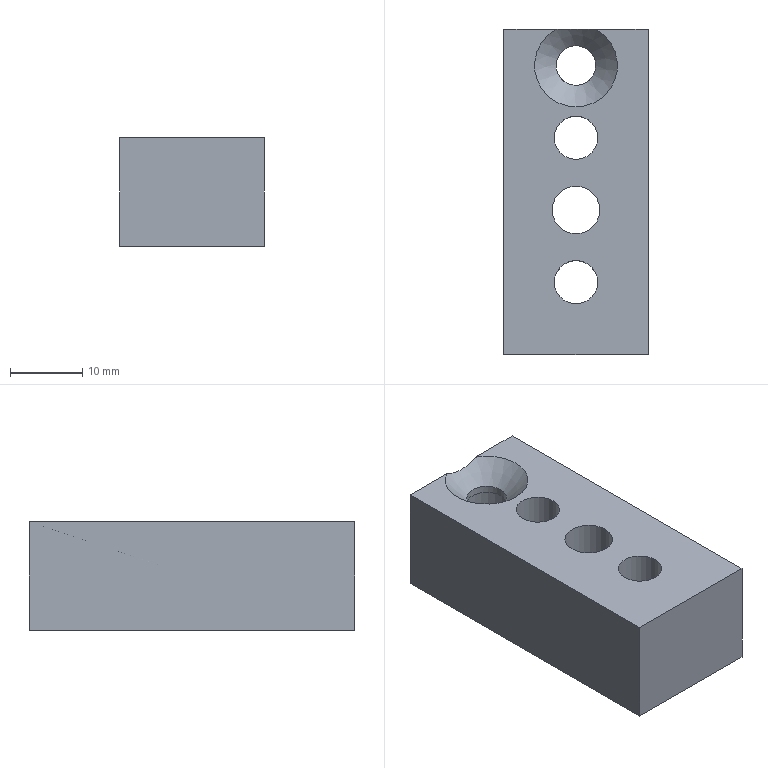Part | NX | features BREP 1 | 1 solid | 15 faces | box 20 x 45 x 15 mm | volume 10997 mm3 | plane 8 | cylinder 6 | cone 1 | commonest cylinder face diameters 6 x2 5.5 x1 6.6 x1 8 x1 11 x1
STEP:
#1=CARTESIAN_POINT('',(-3.,7.5,7.5));
#2=VERTEX_POINT('',#1);
#3=CARTESIAN_POINT('',(0.,7.5,7.5));
#4=DIRECTION('',(0.,0.,-1.));
#5=DIRECTION('',(-1.,0.,0.));
#6=AXIS2_PLACEMENT_3D('',#3,#4,#5);
#7=CIRCLE('',#6,3.);
#8=EDGE_CURVE('',#2,#2,#7,.T.);
#9=ORIENTED_EDGE('',*,*,#8,.T.);
#10=EDGE_LOOP('',(#9));
#11=FACE_BOUND('',#10,.T.);
#12=CARTESIAN_POINT('',(-3.,-12.5,7.5));
#13=VERTEX_POINT('',#12);
#14=CARTESIAN_POINT('',(0.,-12.5,7.5));
#15=DIRECTION('',(0.,0.,-1.));
#16=DIRECTION('',(-1.,0.,0.));
#17=AXIS2_PLACEMENT_3D('',#14,#15,#16);
#18=CIRCLE('',#17,3.);
#19=EDGE_CURVE('',#13,#13,#18,.T.);
#20=ORIENTED_EDGE('',*,*,#19,.T.);
#21=EDGE_LOOP('',(#20));
#22=FACE_BOUND('',#21,.T.);
#23=CARTESIAN_POINT('',(-3.3,-2.5,7.5));
#24=VERTEX_POINT('',#23);
#25=CARTESIAN_POINT('',(0.,-2.5,7.5));
#26=DIRECTION('',(0.,0.,-1.));
#27=DIRECTION('',(-1.,0.,0.));
#28=AXIS2_PLACEMENT_3D('',#25,#26,#27);
#29=CIRCLE('',#28,3.3);
#30=EDGE_CURVE('',#24,#24,#29,.T.);
#31=ORIENTED_EDGE('',*,*,#30,.T.);
#32=EDGE_LOOP('',(#31));
#33=FACE_BOUND('',#32,.T.);
#34=CARTESIAN_POINT('',(-2.809,22.5,7.5));
#35=VERTEX_POINT('',#34);
#36=CARTESIAN_POINT('',(2.809,22.5,7.5));
#37=VERTEX_POINT('',#36);
#38=CARTESIAN_POINT('',(0.,17.5,7.5));
#39=DIRECTION('',(0.,0.,1.));
#40=DIRECTION('',(1.,0.,0.));
#41=AXIS2_PLACEMENT_3D('',#38,#39,#40);
#42=CIRCLE('',#41,5.735);
#43=EDGE_CURVE('',#35,#37,#42,.T.);
#44=ORIENTED_EDGE('',*,*,#43,.F.);
#45=CARTESIAN_POINT('',(-10.,22.5,7.5));
#46=VERTEX_POINT('',#45);
#47=CARTESIAN_POINT('',(-10.,22.5,7.5));
#48=DIRECTION('',(-1.,0.,0.));
#49=VECTOR('',#48,1000.);
#50=LINE('',#47,#49);
#51=EDGE_CURVE('',#35,#46,#50,.T.);
#52=ORIENTED_EDGE('',*,*,#51,.T.);
#53=CARTESIAN_POINT('',(-10.,-22.5,7.5));
#54=VERTEX_POINT('',#53);
#55=CARTESIAN_POINT('',(-10.,-22.5,7.5));
#56=DIRECTION('',(0.,-1.,0.));
#57=VECTOR('',#56,1000.);
#58=LINE('',#55,#57);
#59=EDGE_CURVE('',#46,#54,#58,.T.);
#60=ORIENTED_EDGE('',*,*,#59,.T.);
#61=CARTESIAN_POINT('',(10.,-22.5,7.5));
#62=VERTEX_POINT('',#61);
#63=CARTESIAN_POINT('',(-10.,-22.5,7.5));
#64=DIRECTION('',(1.,0.,0.));
#65=VECTOR('',#64,1000.);
#66=LINE('',#63,#65);
#67=EDGE_CURVE('',#54,#62,#66,.T.);
#68=ORIENTED_EDGE('',*,*,#67,.T.);
#69=CARTESIAN_POINT('',(10.,22.5,7.5));
#70=VERTEX_POINT('',#69);
#71=CARTESIAN_POINT('',(10.,-22.5,7.5));
#72=DIRECTION('',(0.,1.,0.));
#73=VECTOR('',#72,1000.);
#74=LINE('',#71,#73);
#75=EDGE_CURVE('',#62,#70,#74,.T.);
#76=ORIENTED_EDGE('',*,*,#75,.T.);
#77=CARTESIAN_POINT('',(-10.,22.5,7.5));
#78=DIRECTION('',(-1.,0.,0.));
#79=VECTOR('',#78,1000.);
#80=LINE('',#77,#79);
#81=EDGE_CURVE('',#70,#37,#80,.T.);
#82=ORIENTED_EDGE('',*,*,#81,.T.);
#83=EDGE_LOOP('',(#44,#52,#60,#68,#76,#82));
#84=FACE_BOUND('',#83,.T.);
#85=CARTESIAN_POINT('',(0.,0.,7.5));
#86=DIRECTION('',(0.,0.,-1.));
#87=DIRECTION('',(1.,0.,0.));
#88=AXIS2_PLACEMENT_3D('',#85,#86,#87);
#89=PLANE('',#88);
#90=ADVANCED_FACE('',(#11,#22,#33,#84),#89,.F.);
#91=CARTESIAN_POINT('',(10.,-22.5,-7.5));
#92=VERTEX_POINT('',#91);
#93=CARTESIAN_POINT('',(10.,22.5,-7.5));
#94=VERTEX_POINT('',#93);
#95=CARTESIAN_POINT('',(10.,-22.5,-7.5));
#96=DIRECTION('',(0.,1.,0.));
#97=VECTOR('',#96,1000.);
#98=LINE('',#95,#97);
#99=EDGE_CURVE('',#92,#94,#98,.T.);
#100=ORIENTED_EDGE('',*,*,#99,.T.);
#101=CARTESIAN_POINT('',(10.,22.5,7.5));
#102=DIRECTION('',(0.,0.,-1.));
#103=VECTOR('',#102,1000.);
#104=LINE('',#101,#103);
#105=EDGE_CURVE('',#70,#94,#104,.T.);
#106=ORIENTED_EDGE('',*,*,#105,.F.);
#107=ORIENTED_EDGE('',*,*,#75,.F.);
#108=CARTESIAN_POINT('',(10.,-22.5,7.5));
#109=DIRECTION('',(0.,0.,-1.));
#110=VECTOR('',#109,1000.);
#111=LINE('',#108,#110);
#112=EDGE_CURVE('',#62,#92,#111,.T.);
#113=ORIENTED_EDGE('',*,*,#112,.T.);
#114=EDGE_LOOP('',(#100,#106,#107,#113));
#115=FACE_BOUND('',#114,.T.);
#116=CARTESIAN_POINT('',(10.,-22.5,7.5));
#117=DIRECTION('',(-1.,0.,0.));
#118=DIRECTION('',(0.,0.,-1.));
#119=AXIS2_PLACEMENT_3D('',#116,#117,#118);
#120=PLANE('',#119);
#121=ADVANCED_FACE('',(#115),#120,.F.);
#122=ORIENTED_EDGE('',*,*,#51,.F.);
#123=CARTESIAN_POINT('',(-2.809,22.5,7.5));
#124=CARTESIAN_POINT('',(-1.929,22.5,7.069));
#125=CARTESIAN_POINT('',(-0.01669,22.5,6.462));
#126=CARTESIAN_POINT('',(1.924,22.5,7.067));
#127=CARTESIAN_POINT('',(2.809,22.5,7.5));
#128=B_SPLINE_CURVE_WITH_KNOTS('',3,(#123,#124,#125,#126,#127),.UNSPECIFIED.,.F.,.F.,(4,1,4),(0.,0.002898,0.005795),.UNSPECIFIED.);
#129=EDGE_CURVE('',#35,#37,#128,.T.);
#130=ORIENTED_EDGE('',*,*,#129,.T.);
#131=ORIENTED_EDGE('',*,*,#81,.F.);
#132=ORIENTED_EDGE('',*,*,#105,.T.);
#133=CARTESIAN_POINT('',(-10.,22.5,-7.5));
#134=VERTEX_POINT('',#133);
#135=CARTESIAN_POINT('',(-10.,22.5,-7.5));
#136=DIRECTION('',(-1.,0.,0.));
#137=VECTOR('',#136,1000.);
#138=LINE('',#135,#137);
#139=EDGE_CURVE('',#94,#134,#138,.T.);
#140=ORIENTED_EDGE('',*,*,#139,.T.);
#141=CARTESIAN_POINT('',(-10.,22.5,7.5));
#142=DIRECTION('',(0.,0.,-1.));
#143=VECTOR('',#142,1000.);
#144=LINE('',#141,#143);
#145=EDGE_CURVE('',#46,#134,#144,.T.);
#146=ORIENTED_EDGE('',*,*,#145,.F.);
#147=EDGE_LOOP('',(#122,#130,#131,#132,#140,#146));
#148=FACE_BOUND('',#147,.T.);
#149=CARTESIAN_POINT('',(-10.,22.5,7.5));
#150=DIRECTION('',(0.,-1.,0.));
#151=DIRECTION('',(0.,0.,1.));
#152=AXIS2_PLACEMENT_3D('',#149,#150,#151);
#153=PLANE('',#152);
#154=ADVANCED_FACE('',(#148),#153,.F.);
#155=CARTESIAN_POINT('',(-10.,-22.5,-7.5));
#156=VERTEX_POINT('',#155);
#157=CARTESIAN_POINT('',(-10.,-22.5,-7.5));
#158=DIRECTION('',(0.,-1.,0.));
#159=VECTOR('',#158,1000.);
#160=LINE('',#157,#159);
#161=EDGE_CURVE('',#134,#156,#160,.T.);
#162=ORIENTED_EDGE('',*,*,#161,.T.);
#163=CARTESIAN_POINT('',(-10.,-22.5,7.5));
#164=DIRECTION('',(0.,0.,-1.));
#165=VECTOR('',#164,1000.);
#166=LINE('',#163,#165);
#167=EDGE_CURVE('',#54,#156,#166,.T.);
#168=ORIENTED_EDGE('',*,*,#167,.F.);
#169=ORIENTED_EDGE('',*,*,#59,.F.);
#170=ORIENTED_EDGE('',*,*,#145,.T.);
#171=EDGE_LOOP('',(#162,#168,#169,#170));
#172=FACE_BOUND('',#171,.T.);
#173=CARTESIAN_POINT('',(-10.,-22.5,7.5));
#174=DIRECTION('',(1.,0.,0.));
#175=DIRECTION('',(0.,0.,1.));
#176=AXIS2_PLACEMENT_3D('',#173,#174,#175);
#177=PLANE('',#176);
#178=ADVANCED_FACE('',(#172),#177,.F.);
#179=CARTESIAN_POINT('',(-10.,-22.5,-7.5));
#180=DIRECTION('',(1.,0.,0.));
#181=VECTOR('',#180,1000.);
#182=LINE('',#179,#181);
#183=EDGE_CURVE('',#156,#92,#182,.T.);
#184=ORIENTED_EDGE('',*,*,#183,.T.);
#185=ORIENTED_EDGE('',*,*,#112,.F.);
#186=ORIENTED_EDGE('',*,*,#67,.F.);
#187=ORIENTED_EDGE('',*,*,#167,.T.);
#188=EDGE_LOOP('',(#184,#185,#186,#187));
#189=FACE_BOUND('',#188,.T.);
#190=CARTESIAN_POINT('',(-10.,-22.5,7.5));
#191=DIRECTION('',(0.,1.,0.));
#192=DIRECTION('',(0.,0.,-1.));
#193=AXIS2_PLACEMENT_3D('',#190,#191,#192);
#194=PLANE('',#193);
#195=ADVANCED_FACE('',(#189),#194,.F.);
#196=CARTESIAN_POINT('',(-3.,7.5,-7.5));
#197=VERTEX_POINT('',#196);
#198=CARTESIAN_POINT('',(0.,7.5,-7.5));
#199=DIRECTION('',(0.,0.,-1.));
#200=DIRECTION('',(-1.,0.,0.));
#201=AXIS2_PLACEMENT_3D('',#198,#199,#200);
#202=CIRCLE('',#201,3.);
#203=EDGE_CURVE('',#197,#197,#202,.T.);
#204=ORIENTED_EDGE('',*,*,#203,.F.);
#205=EDGE_LOOP('',(#204));
#206=FACE_BOUND('',#205,.T.);
#207=CARTESIAN_POINT('',(-3.,-12.5,-7.5));
#208=VERTEX_POINT('',#207);
#209=CARTESIAN_POINT('',(0.,-12.5,-7.5));
#210=DIRECTION('',(0.,0.,-1.));
#211=DIRECTION('',(-1.,0.,0.));
#212=AXIS2_PLACEMENT_3D('',#209,#210,#211);
#213=CIRCLE('',#212,3.);
#214=EDGE_CURVE('',#208,#208,#213,.T.);
#215=ORIENTED_EDGE('',*,*,#214,.F.);
#216=EDGE_LOOP('',(#215));
#217=FACE_BOUND('',#216,.T.);
#218=CARTESIAN_POINT('',(-5.5,-2.5,-7.5));
#219=VERTEX_POINT('',#218);
#220=CARTESIAN_POINT('',(0.,-2.5,-7.5));
#221=DIRECTION('',(0.,0.,-1.));
#222=DIRECTION('',(-1.,0.,0.));
#223=AXIS2_PLACEMENT_3D('',#220,#221,#222);
#224=CIRCLE('',#223,5.5);
#225=EDGE_CURVE('',#219,#219,#224,.T.);
#226=ORIENTED_EDGE('',*,*,#225,.F.);
#227=EDGE_LOOP('',(#226));
#228=FACE_BOUND('',#227,.T.);
#229=CARTESIAN_POINT('',(-4.,17.5,-7.5));
#230=VERTEX_POINT('',#229);
#231=CARTESIAN_POINT('',(0.,17.5,-7.5));
#232=DIRECTION('',(0.,0.,-1.));
#233=DIRECTION('',(-1.,0.,0.));
#234=AXIS2_PLACEMENT_3D('',#231,#232,#233);
#235=CIRCLE('',#234,4.);
#236=EDGE_CURVE('',#230,#230,#235,.T.);
#237=ORIENTED_EDGE('',*,*,#236,.F.);
#238=EDGE_LOOP('',(#237));
#239=FACE_BOUND('',#238,.T.);
#240=ORIENTED_EDGE('',*,*,#99,.F.);
#241=ORIENTED_EDGE('',*,*,#183,.F.);
#242=ORIENTED_EDGE('',*,*,#161,.F.);
#243=ORIENTED_EDGE('',*,*,#139,.F.);
#244=EDGE_LOOP('',(#240,#241,#242,#243));
#245=FACE_BOUND('',#244,.T.);
#246=CARTESIAN_POINT('',(0.,0.,-7.5));
#247=DIRECTION('',(0.,0.,-1.));
#248=DIRECTION('',(1.,0.,0.));
#249=AXIS2_PLACEMENT_3D('',#246,#247,#248);
#250=PLANE('',#249);
#251=ADVANCED_FACE('',(#206,#217,#228,#239,#245),#250,.T.);
#252=CARTESIAN_POINT('',(2.75,17.5,4.515));
#253=VERTEX_POINT('',#252);
#254=CARTESIAN_POINT('',(0.,17.5,4.515));
#255=DIRECTION('',(0.,0.,1.));
#256=DIRECTION('',(1.,0.,0.));
#257=AXIS2_PLACEMENT_3D('',#254,#255,#256);
#258=CIRCLE('',#257,2.75);
#259=EDGE_CURVE('',#253,#253,#258,.T.);
#260=ORIENTED_EDGE('',*,*,#259,.F.);
#261=EDGE_LOOP('',(#260));
#262=FACE_BOUND('',#261,.T.);
#263=ORIENTED_EDGE('',*,*,#43,.T.);
#264=ORIENTED_EDGE('',*,*,#129,.F.);
#265=EDGE_LOOP('',(#263,#264));
#266=FACE_BOUND('',#265,.T.);
#267=CARTESIAN_POINT('',(0.,17.5,7.5));
#268=DIRECTION('',(0.,0.,1.));
#269=DIRECTION('',(-1.,0.,0.));
#270=AXIS2_PLACEMENT_3D('',#267,#268,#269);
#271=CONICAL_SURFACE('',#270,5.735,0.7854);
#272=ADVANCED_FACE('',(#262,#266),#271,.F.);
#273=CARTESIAN_POINT('',(2.75,17.5,3.5));
#274=VERTEX_POINT('',#273);
#275=CARTESIAN_POINT('',(0.,17.5,3.5));
#276=DIRECTION('',(0.,0.,-1.));
#277=DIRECTION('',(1.,0.,0.));
#278=AXIS2_PLACEMENT_3D('',#275,#276,#277);
#279=CIRCLE('',#278,2.75);
#280=EDGE_CURVE('',#274,#274,#279,.T.);
#281=ORIENTED_EDGE('',*,*,#280,.T.);
#282=EDGE_LOOP('',(#281));
#283=FACE_BOUND('',#282,.T.);
#284=ORIENTED_EDGE('',*,*,#259,.T.);
#285=EDGE_LOOP('',(#284));
#286=FACE_BOUND('',#285,.T.);
#287=CARTESIAN_POINT('',(0.,17.5,7.5));
#288=DIRECTION('',(0.,0.,1.));
#289=DIRECTION('',(-1.,0.,0.));
#290=AXIS2_PLACEMENT_3D('',#287,#288,#289);
#291=CYLINDRICAL_SURFACE('',#290,2.75);
#292=ADVANCED_FACE('',(#283,#286),#291,.F.);
#293=CARTESIAN_POINT('',(-4.,17.5,3.5));
#294=VERTEX_POINT('',#293);
#295=CARTESIAN_POINT('',(0.,17.5,3.5));
#296=DIRECTION('',(0.,0.,-1.));
#297=DIRECTION('',(-1.,0.,0.));
#298=AXIS2_PLACEMENT_3D('',#295,#296,#297);
#299=CIRCLE('',#298,4.);
#300=EDGE_CURVE('',#294,#294,#299,.T.);
#301=ORIENTED_EDGE('',*,*,#300,.T.);
#302=EDGE_LOOP('',(#301));
#303=FACE_BOUND('',#302,.T.);
#304=ORIENTED_EDGE('',*,*,#280,.F.);
#305=EDGE_LOOP('',(#304));
#306=FACE_BOUND('',#305,.T.);
#307=CARTESIAN_POINT('',(0.,17.5,3.5));
#308=DIRECTION('',(0.,0.,1.));
#309=DIRECTION('',(-1.,0.,0.));
#310=AXIS2_PLACEMENT_3D('',#307,#308,#309);
#311=PLANE('',#310);
#312=ADVANCED_FACE('',(#303,#306),#311,.F.);
#313=ORIENTED_EDGE('',*,*,#300,.F.);
#314=EDGE_LOOP('',(#313));
#315=FACE_BOUND('',#314,.T.);
#316=ORIENTED_EDGE('',*,*,#236,.T.);
#317=EDGE_LOOP('',(#316));
#318=FACE_BOUND('',#317,.T.);
#319=CARTESIAN_POINT('',(0.,17.5,-7.5));
#320=DIRECTION('',(0.,0.,-1.));
#321=DIRECTION('',(1.,0.,0.));
#322=AXIS2_PLACEMENT_3D('',#319,#320,#321);
#323=CYLINDRICAL_SURFACE('',#322,4.);
#324=ADVANCED_FACE('',(#315,#318),#323,.F.);
#325=ORIENTED_EDGE('',*,*,#30,.F.);
#326=EDGE_LOOP('',(#325));
#327=FACE_BOUND('',#326,.T.);
#328=CARTESIAN_POINT('',(-3.3,-2.5,-1.1));
#329=VERTEX_POINT('',#328);
#330=CARTESIAN_POINT('',(0.,-2.5,-1.1));
#331=DIRECTION('',(0.,0.,-1.));
#332=DIRECTION('',(-1.,0.,0.));
#333=AXIS2_PLACEMENT_3D('',#330,#331,#332);
#334=CIRCLE('',#333,3.3);
#335=EDGE_CURVE('',#329,#329,#334,.T.);
#336=ORIENTED_EDGE('',*,*,#335,.T.);
#337=EDGE_LOOP('',(#336));
#338=FACE_BOUND('',#337,.T.);
#339=CARTESIAN_POINT('',(0.,-2.5,-7.5));
#340=DIRECTION('',(0.,0.,-1.));
#341=DIRECTION('',(1.,0.,0.));
#342=AXIS2_PLACEMENT_3D('',#339,#340,#341);
#343=CYLINDRICAL_SURFACE('',#342,3.3);
#344=ADVANCED_FACE('',(#327,#338),#343,.F.);
#345=ORIENTED_EDGE('',*,*,#335,.F.);
#346=EDGE_LOOP('',(#345));
#347=FACE_BOUND('',#346,.T.);
#348=CARTESIAN_POINT('',(-5.5,-2.5,-1.1));
#349=VERTEX_POINT('',#348);
#350=CARTESIAN_POINT('',(0.,-2.5,-1.1));
#351=DIRECTION('',(0.,0.,-1.));
#352=DIRECTION('',(-1.,0.,0.));
#353=AXIS2_PLACEMENT_3D('',#350,#351,#352);
#354=CIRCLE('',#353,5.5);
#355=EDGE_CURVE('',#349,#349,#354,.T.);
#356=ORIENTED_EDGE('',*,*,#355,.T.);
#357=EDGE_LOOP('',(#356));
#358=FACE_BOUND('',#357,.T.);
#359=CARTESIAN_POINT('',(3.3,-2.5,-1.1));
#360=DIRECTION('',(0.,0.,1.));
#361=DIRECTION('',(-1.,0.,0.));
#362=AXIS2_PLACEMENT_3D('',#359,#360,#361);
#363=PLANE('',#362);
#364=ADVANCED_FACE('',(#347,#358),#363,.F.);
#365=ORIENTED_EDGE('',*,*,#355,.F.);
#366=EDGE_LOOP('',(#365));
#367=FACE_BOUND('',#366,.T.);
#368=ORIENTED_EDGE('',*,*,#225,.T.);
#369=EDGE_LOOP('',(#368));
#370=FACE_BOUND('',#369,.T.);
#371=CARTESIAN_POINT('',(0.,-2.5,-7.5));
#372=DIRECTION('',(0.,0.,-1.));
#373=DIRECTION('',(1.,0.,0.));
#374=AXIS2_PLACEMENT_3D('',#371,#372,#373);
#375=CYLINDRICAL_SURFACE('',#374,5.5);
#376=ADVANCED_FACE('',(#367,#370),#375,.F.);
#377=ORIENTED_EDGE('',*,*,#19,.F.);
#378=EDGE_LOOP('',(#377));
#379=FACE_BOUND('',#378,.T.);
#380=ORIENTED_EDGE('',*,*,#214,.T.);
#381=EDGE_LOOP('',(#380));
#382=FACE_BOUND('',#381,.T.);
#383=CARTESIAN_POINT('',(0.,-12.5,-7.5));
#384=DIRECTION('',(0.,0.,-1.));
#385=DIRECTION('',(1.,0.,0.));
#386=AXIS2_PLACEMENT_3D('',#383,#384,#385);
#387=CYLINDRICAL_SURFACE('',#386,3.);
#388=ADVANCED_FACE('',(#379,#382),#387,.F.);
#389=ORIENTED_EDGE('',*,*,#8,.F.);
#390=EDGE_LOOP('',(#389));
#391=FACE_BOUND('',#390,.T.);
#392=ORIENTED_EDGE('',*,*,#203,.T.);
#393=EDGE_LOOP('',(#392));
#394=FACE_BOUND('',#393,.T.);
#395=CARTESIAN_POINT('',(0.,7.5,-7.5));
#396=DIRECTION('',(0.,0.,-1.));
#397=DIRECTION('',(1.,0.,0.));
#398=AXIS2_PLACEMENT_3D('',#395,#396,#397);
#399=CYLINDRICAL_SURFACE('',#398,3.);
#400=ADVANCED_FACE('',(#391,#394),#399,.F.);
#401=CLOSED_SHELL('',(#90,#121,#154,#178,#195,#251,#272,#292,#312,#324,#344,#364,#376,#388,#400));
#402=MANIFOLD_SOLID_BREP('',#401);
#403=(LENGTH_UNIT()NAMED_UNIT(*)SI_UNIT(.MILLI.,.METRE.));
#404=UNCERTAINTY_MEASURE_WITH_UNIT(LENGTH_MEASURE(0.0508),#403,'','');
#405=(NAMED_UNIT(*)PLANE_ANGLE_UNIT()SI_UNIT($,.RADIAN.));
#406=(NAMED_UNIT(*)SI_UNIT($,.STERADIAN.)SOLID_ANGLE_UNIT());
#407=(GEOMETRIC_REPRESENTATION_CONTEXT(3)GLOBAL_UNCERTAINTY_ASSIGNED_CONTEXT((#404))GLOBAL_UNIT_ASSIGNED_CONTEXT((#403,#405,#406))REPRESENTATION_CONTEXT('',''));
#408=ADVANCED_BREP_SHAPE_REPRESENTATION('',(#402),#407);